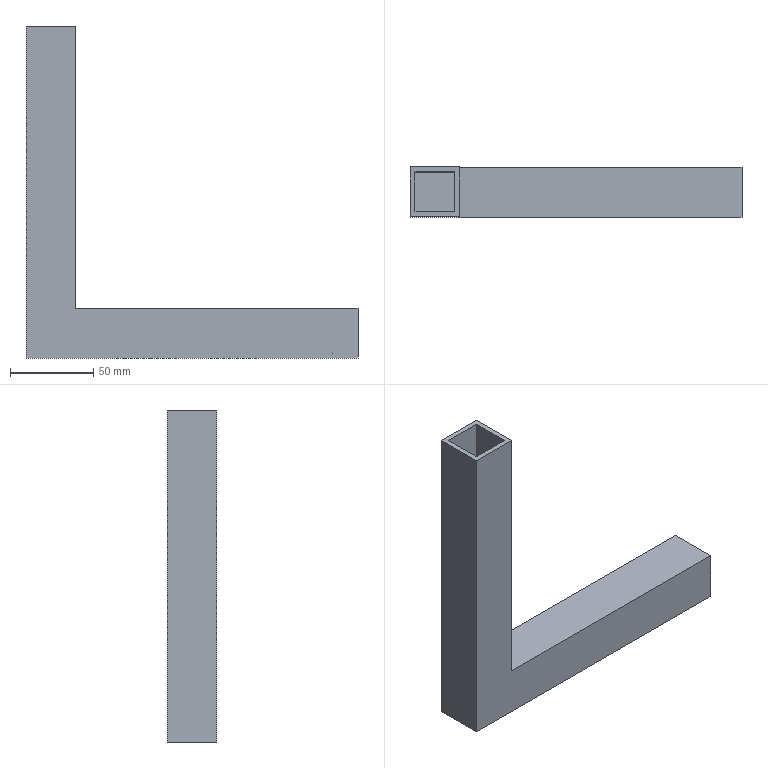Part | SolidWorks | features Extrusion 1, ICE 1, Shell 1 | 1 solid | 14 faces | box 200 x 30 x 200 mm | volume 119880 mm3 | plane 14
STEP:
#1=CARTESIAN_POINT('',(200.,0.,0.));
#2=VERTEX_POINT('',#1);
#3=CARTESIAN_POINT('',(200.,30.,0.));
#4=VERTEX_POINT('',#3);
#5=CARTESIAN_POINT('',(200.,30.,0.));
#6=DIRECTION('',(0.,1.,0.));
#7=VECTOR('',#6,1000.);
#8=LINE('',#5,#7);
#9=EDGE_CURVE('',#2,#4,#8,.T.);
#10=ORIENTED_EDGE('',*,*,#9,.F.);
#11=CARTESIAN_POINT('',(200.,0.,-30.));
#12=VERTEX_POINT('',#11);
#13=CARTESIAN_POINT('',(200.,0.,-30.));
#14=DIRECTION('',(0.,0.,1.));
#15=VECTOR('',#14,1000.);
#16=LINE('',#13,#15);
#17=EDGE_CURVE('',#12,#2,#16,.T.);
#18=ORIENTED_EDGE('',*,*,#17,.F.);
#19=CARTESIAN_POINT('',(200.,30.,-30.));
#20=VERTEX_POINT('',#19);
#21=CARTESIAN_POINT('',(200.,30.,-30.));
#22=DIRECTION('',(0.,1.,0.));
#23=VECTOR('',#22,1000.);
#24=LINE('',#21,#23);
#25=EDGE_CURVE('',#12,#20,#24,.T.);
#26=ORIENTED_EDGE('',*,*,#25,.T.);
#27=CARTESIAN_POINT('',(200.,30.,-30.));
#28=DIRECTION('',(0.,0.,1.));
#29=VECTOR('',#28,1000.);
#30=LINE('',#27,#29);
#31=EDGE_CURVE('',#20,#4,#30,.T.);
#32=ORIENTED_EDGE('',*,*,#31,.T.);
#33=EDGE_LOOP('',(#10,#18,#26,#32));
#34=FACE_OUTER_BOUND('',#33,.T.);
#35=CARTESIAN_POINT('',(200.,3.,-27.));
#36=VERTEX_POINT('',#35);
#37=CARTESIAN_POINT('',(200.,3.,-3.));
#38=VERTEX_POINT('',#37);
#39=CARTESIAN_POINT('',(200.,3.,-30.));
#40=DIRECTION('',(0.,0.,1.));
#41=VECTOR('',#40,1000.);
#42=LINE('',#39,#41);
#43=EDGE_CURVE('',#36,#38,#42,.T.);
#44=ORIENTED_EDGE('',*,*,#43,.T.);
#45=CARTESIAN_POINT('',(200.,27.,-3.));
#46=VERTEX_POINT('',#45);
#47=CARTESIAN_POINT('',(200.,30.,-3.));
#48=DIRECTION('',(0.,1.,0.));
#49=VECTOR('',#48,1000.);
#50=LINE('',#47,#49);
#51=EDGE_CURVE('',#38,#46,#50,.T.);
#52=ORIENTED_EDGE('',*,*,#51,.T.);
#53=CARTESIAN_POINT('',(200.,27.,-27.));
#54=VERTEX_POINT('',#53);
#55=CARTESIAN_POINT('',(200.,27.,-30.));
#56=DIRECTION('',(0.,0.,1.));
#57=VECTOR('',#56,1000.);
#58=LINE('',#55,#57);
#59=EDGE_CURVE('',#54,#46,#58,.T.);
#60=ORIENTED_EDGE('',*,*,#59,.F.);
#61=CARTESIAN_POINT('',(200.,30.,-27.));
#62=DIRECTION('',(0.,1.,0.));
#63=VECTOR('',#62,1000.);
#64=LINE('',#61,#63);
#65=EDGE_CURVE('',#36,#54,#64,.T.);
#66=ORIENTED_EDGE('',*,*,#65,.F.);
#67=EDGE_LOOP('',(#44,#52,#60,#66));
#68=FACE_BOUND('',#67,.T.);
#69=CARTESIAN_POINT('',(200.,30.,-30.));
#70=DIRECTION('',(1.,0.,0.));
#71=DIRECTION('',(0.,0.,-1.));
#72=AXIS2_PLACEMENT_3D('',#69,#70,#71);
#73=PLANE('',#72);
#74=ADVANCED_FACE('',(#34,#68),#73,.T.);
#75=CARTESIAN_POINT('',(0.,30.,170.));
#76=VERTEX_POINT('',#75);
#77=CARTESIAN_POINT('',(0.,0.,170.));
#78=VERTEX_POINT('',#77);
#79=CARTESIAN_POINT('',(0.,0.,170.));
#80=DIRECTION('',(0.,-1.,0.));
#81=VECTOR('',#80,1000.);
#82=LINE('',#79,#81);
#83=EDGE_CURVE('',#76,#78,#82,.T.);
#84=ORIENTED_EDGE('',*,*,#83,.T.);
#85=CARTESIAN_POINT('',(30.,0.,170.));
#86=VERTEX_POINT('',#85);
#87=CARTESIAN_POINT('',(30.,0.,170.));
#88=DIRECTION('',(1.,0.,0.));
#89=VECTOR('',#88,1000.);
#90=LINE('',#87,#89);
#91=EDGE_CURVE('',#78,#86,#90,.T.);
#92=ORIENTED_EDGE('',*,*,#91,.T.);
#93=CARTESIAN_POINT('',(30.,30.,170.));
#94=VERTEX_POINT('',#93);
#95=CARTESIAN_POINT('',(30.,30.,170.));
#96=DIRECTION('',(0.,1.,0.));
#97=VECTOR('',#96,1000.);
#98=LINE('',#95,#97);
#99=EDGE_CURVE('',#86,#94,#98,.T.);
#100=ORIENTED_EDGE('',*,*,#99,.T.);
#101=CARTESIAN_POINT('',(0.,30.,170.));
#102=DIRECTION('',(-1.,0.,0.));
#103=VECTOR('',#102,1000.);
#104=LINE('',#101,#103);
#105=EDGE_CURVE('',#94,#76,#104,.T.);
#106=ORIENTED_EDGE('',*,*,#105,.T.);
#107=EDGE_LOOP('',(#84,#92,#100,#106));
#108=FACE_OUTER_BOUND('',#107,.T.);
#109=CARTESIAN_POINT('',(3.,27.,170.));
#110=VERTEX_POINT('',#109);
#111=CARTESIAN_POINT('',(3.,3.,170.));
#112=VERTEX_POINT('',#111);
#113=CARTESIAN_POINT('',(3.,0.,170.));
#114=DIRECTION('',(0.,-1.,0.));
#115=VECTOR('',#114,1000.);
#116=LINE('',#113,#115);
#117=EDGE_CURVE('',#110,#112,#116,.T.);
#118=ORIENTED_EDGE('',*,*,#117,.F.);
#119=CARTESIAN_POINT('',(27.,27.,170.));
#120=VERTEX_POINT('',#119);
#121=CARTESIAN_POINT('',(0.,27.,170.));
#122=DIRECTION('',(-1.,0.,0.));
#123=VECTOR('',#122,1000.);
#124=LINE('',#121,#123);
#125=EDGE_CURVE('',#120,#110,#124,.T.);
#126=ORIENTED_EDGE('',*,*,#125,.F.);
#127=CARTESIAN_POINT('',(27.,3.,170.));
#128=VERTEX_POINT('',#127);
#129=CARTESIAN_POINT('',(27.,0.,170.));
#130=DIRECTION('',(0.,1.,0.));
#131=VECTOR('',#130,1000.);
#132=LINE('',#129,#131);
#133=EDGE_CURVE('',#128,#120,#132,.T.);
#134=ORIENTED_EDGE('',*,*,#133,.F.);
#135=CARTESIAN_POINT('',(200.,3.,170.));
#136=DIRECTION('',(1.,0.,0.));
#137=VECTOR('',#136,1000.);
#138=LINE('',#135,#137);
#139=EDGE_CURVE('',#112,#128,#138,.T.);
#140=ORIENTED_EDGE('',*,*,#139,.F.);
#141=EDGE_LOOP('',(#118,#126,#134,#140));
#142=FACE_BOUND('',#141,.T.);
#143=CARTESIAN_POINT('',(0.,0.,170.));
#144=DIRECTION('',(0.,0.,-1.));
#145=DIRECTION('',(-1.,0.,0.));
#146=AXIS2_PLACEMENT_3D('',#143,#144,#145);
#147=PLANE('',#146);
#148=ADVANCED_FACE('',(#108,#142),#147,.F.);
#149=CARTESIAN_POINT('',(30.,0.,0.));
#150=VERTEX_POINT('',#149);
#151=CARTESIAN_POINT('',(30.,30.,0.));
#152=VERTEX_POINT('',#151);
#153=CARTESIAN_POINT('',(30.,30.,0.));
#154=DIRECTION('',(0.,1.,0.));
#155=VECTOR('',#154,1000.);
#156=LINE('',#153,#155);
#157=EDGE_CURVE('',#150,#152,#156,.T.);
#158=ORIENTED_EDGE('',*,*,#157,.F.);
#159=CARTESIAN_POINT('',(200.,0.,0.));
#160=DIRECTION('',(1.,0.,0.));
#161=VECTOR('',#160,1000.);
#162=LINE('',#159,#161);
#163=EDGE_CURVE('',#150,#2,#162,.T.);
#164=ORIENTED_EDGE('',*,*,#163,.T.);
#165=ORIENTED_EDGE('',*,*,#9,.T.);
#166=CARTESIAN_POINT('',(0.,30.,0.));
#167=DIRECTION('',(-1.,0.,0.));
#168=VECTOR('',#167,1000.);
#169=LINE('',#166,#168);
#170=EDGE_CURVE('',#4,#152,#169,.T.);
#171=ORIENTED_EDGE('',*,*,#170,.T.);
#172=EDGE_LOOP('',(#158,#164,#165,#171));
#173=FACE_OUTER_BOUND('',#172,.T.);
#174=CARTESIAN_POINT('',(0.,0.,0.));
#175=DIRECTION('',(0.,0.,-1.));
#176=DIRECTION('',(-1.,0.,0.));
#177=AXIS2_PLACEMENT_3D('',#174,#175,#176);
#178=PLANE('',#177);
#179=ADVANCED_FACE('',(#173),#178,.F.);
#180=ORIENTED_EDGE('',*,*,#163,.F.);
#181=CARTESIAN_POINT('',(30.,0.,170.));
#182=DIRECTION('',(0.,0.,-1.));
#183=VECTOR('',#182,1000.);
#184=LINE('',#181,#183);
#185=EDGE_CURVE('',#86,#150,#184,.T.);
#186=ORIENTED_EDGE('',*,*,#185,.F.);
#187=ORIENTED_EDGE('',*,*,#91,.F.);
#188=CARTESIAN_POINT('',(0.,0.,-30.));
#189=VERTEX_POINT('',#188);
#190=CARTESIAN_POINT('',(0.,0.,-30.));
#191=DIRECTION('',(0.,0.,1.));
#192=VECTOR('',#191,1000.);
#193=LINE('',#190,#192);
#194=EDGE_CURVE('',#189,#78,#193,.T.);
#195=ORIENTED_EDGE('',*,*,#194,.F.);
#196=CARTESIAN_POINT('',(200.,0.,-30.));
#197=DIRECTION('',(1.,0.,0.));
#198=VECTOR('',#197,1000.);
#199=LINE('',#196,#198);
#200=EDGE_CURVE('',#189,#12,#199,.T.);
#201=ORIENTED_EDGE('',*,*,#200,.T.);
#202=ORIENTED_EDGE('',*,*,#17,.T.);
#203=EDGE_LOOP('',(#180,#186,#187,#195,#201,#202));
#204=FACE_OUTER_BOUND('',#203,.T.);
#205=CARTESIAN_POINT('',(200.,0.,-30.));
#206=DIRECTION('',(0.,-1.,0.));
#207=DIRECTION('',(0.,0.,-1.));
#208=AXIS2_PLACEMENT_3D('',#205,#206,#207);
#209=PLANE('',#208);
#210=ADVANCED_FACE('',(#204),#209,.T.);
#211=ORIENTED_EDGE('',*,*,#194,.T.);
#212=ORIENTED_EDGE('',*,*,#83,.F.);
#213=CARTESIAN_POINT('',(0.,30.,-30.));
#214=VERTEX_POINT('',#213);
#215=CARTESIAN_POINT('',(0.,30.,-30.));
#216=DIRECTION('',(0.,0.,1.));
#217=VECTOR('',#216,1000.);
#218=LINE('',#215,#217);
#219=EDGE_CURVE('',#214,#76,#218,.T.);
#220=ORIENTED_EDGE('',*,*,#219,.F.);
#221=CARTESIAN_POINT('',(0.,0.,-30.));
#222=DIRECTION('',(0.,-1.,0.));
#223=VECTOR('',#222,1000.);
#224=LINE('',#221,#223);
#225=EDGE_CURVE('',#214,#189,#224,.T.);
#226=ORIENTED_EDGE('',*,*,#225,.T.);
#227=EDGE_LOOP('',(#211,#212,#220,#226));
#228=FACE_OUTER_BOUND('',#227,.T.);
#229=CARTESIAN_POINT('',(0.,0.,-30.));
#230=DIRECTION('',(-1.,0.,0.));
#231=DIRECTION('',(0.,0.,1.));
#232=AXIS2_PLACEMENT_3D('',#229,#230,#231);
#233=PLANE('',#232);
#234=ADVANCED_FACE('',(#228),#233,.T.);
#235=ORIENTED_EDGE('',*,*,#170,.F.);
#236=ORIENTED_EDGE('',*,*,#31,.F.);
#237=CARTESIAN_POINT('',(0.,30.,-30.));
#238=DIRECTION('',(-1.,0.,0.));
#239=VECTOR('',#238,1000.);
#240=LINE('',#237,#239);
#241=EDGE_CURVE('',#20,#214,#240,.T.);
#242=ORIENTED_EDGE('',*,*,#241,.T.);
#243=ORIENTED_EDGE('',*,*,#219,.T.);
#244=ORIENTED_EDGE('',*,*,#105,.F.);
#245=CARTESIAN_POINT('',(30.,30.,170.));
#246=DIRECTION('',(0.,0.,-1.));
#247=VECTOR('',#246,1000.);
#248=LINE('',#245,#247);
#249=EDGE_CURVE('',#94,#152,#248,.T.);
#250=ORIENTED_EDGE('',*,*,#249,.T.);
#251=EDGE_LOOP('',(#235,#236,#242,#243,#244,#250));
#252=FACE_OUTER_BOUND('',#251,.T.);
#253=CARTESIAN_POINT('',(0.,30.,-30.));
#254=DIRECTION('',(0.,1.,0.));
#255=DIRECTION('',(0.,0.,1.));
#256=AXIS2_PLACEMENT_3D('',#253,#254,#255);
#257=PLANE('',#256);
#258=ADVANCED_FACE('',(#252),#257,.T.);
#259=ORIENTED_EDGE('',*,*,#200,.F.);
#260=ORIENTED_EDGE('',*,*,#225,.F.);
#261=ORIENTED_EDGE('',*,*,#241,.F.);
#262=ORIENTED_EDGE('',*,*,#25,.F.);
#263=EDGE_LOOP('',(#259,#260,#261,#262));
#264=FACE_OUTER_BOUND('',#263,.T.);
#265=CARTESIAN_POINT('',(0.,0.,-30.));
#266=DIRECTION('',(0.,0.,-1.));
#267=DIRECTION('',(-1.,0.,0.));
#268=AXIS2_PLACEMENT_3D('',#265,#266,#267);
#269=PLANE('',#268);
#270=ADVANCED_FACE('',(#264),#269,.T.);
#271=ORIENTED_EDGE('',*,*,#157,.T.);
#272=ORIENTED_EDGE('',*,*,#249,.F.);
#273=ORIENTED_EDGE('',*,*,#99,.F.);
#274=ORIENTED_EDGE('',*,*,#185,.T.);
#275=EDGE_LOOP('',(#271,#272,#273,#274));
#276=FACE_OUTER_BOUND('',#275,.T.);
#277=CARTESIAN_POINT('',(30.,30.,170.));
#278=DIRECTION('',(-1.,0.,0.));
#279=DIRECTION('',(0.,0.,1.));
#280=AXIS2_PLACEMENT_3D('',#277,#278,#279);
#281=PLANE('',#280);
#282=ADVANCED_FACE('',(#276),#281,.F.);
#283=CARTESIAN_POINT('',(27.,3.,-3.));
#284=VERTEX_POINT('',#283);
#285=CARTESIAN_POINT('',(27.,27.,-3.));
#286=VERTEX_POINT('',#285);
#287=CARTESIAN_POINT('',(27.,0.,-3.));
#288=DIRECTION('',(0.,1.,0.));
#289=VECTOR('',#288,1000.);
#290=LINE('',#287,#289);
#291=EDGE_CURVE('',#284,#286,#290,.T.);
#292=ORIENTED_EDGE('',*,*,#291,.T.);
#293=CARTESIAN_POINT('',(0.,27.,-3.));
#294=DIRECTION('',(-1.,0.,0.));
#295=VECTOR('',#294,1000.);
#296=LINE('',#293,#295);
#297=EDGE_CURVE('',#46,#286,#296,.T.);
#298=ORIENTED_EDGE('',*,*,#297,.F.);
#299=ORIENTED_EDGE('',*,*,#51,.F.);
#300=CARTESIAN_POINT('',(200.,3.,-3.));
#301=DIRECTION('',(1.,0.,0.));
#302=VECTOR('',#301,1000.);
#303=LINE('',#300,#302);
#304=EDGE_CURVE('',#284,#38,#303,.T.);
#305=ORIENTED_EDGE('',*,*,#304,.F.);
#306=EDGE_LOOP('',(#292,#298,#299,#305));
#307=FACE_OUTER_BOUND('',#306,.T.);
#308=CARTESIAN_POINT('',(0.,0.,-3.));
#309=DIRECTION('',(0.,0.,-1.));
#310=DIRECTION('',(-1.,0.,0.));
#311=AXIS2_PLACEMENT_3D('',#308,#309,#310);
#312=PLANE('',#311);
#313=ADVANCED_FACE('',(#307),#312,.T.);
#314=ORIENTED_EDGE('',*,*,#304,.T.);
#315=ORIENTED_EDGE('',*,*,#43,.F.);
#316=CARTESIAN_POINT('',(3.,3.,-27.));
#317=VERTEX_POINT('',#316);
#318=CARTESIAN_POINT('',(200.,3.,-27.));
#319=DIRECTION('',(1.,0.,0.));
#320=VECTOR('',#319,1000.);
#321=LINE('',#318,#320);
#322=EDGE_CURVE('',#317,#36,#321,.T.);
#323=ORIENTED_EDGE('',*,*,#322,.F.);
#324=CARTESIAN_POINT('',(3.,3.,-30.));
#325=DIRECTION('',(0.,0.,1.));
#326=VECTOR('',#325,1000.);
#327=LINE('',#324,#326);
#328=EDGE_CURVE('',#317,#112,#327,.T.);
#329=ORIENTED_EDGE('',*,*,#328,.T.);
#330=ORIENTED_EDGE('',*,*,#139,.T.);
#331=CARTESIAN_POINT('',(27.,3.,-30.));
#332=DIRECTION('',(0.,0.,-1.));
#333=VECTOR('',#332,1000.);
#334=LINE('',#331,#333);
#335=EDGE_CURVE('',#128,#284,#334,.T.);
#336=ORIENTED_EDGE('',*,*,#335,.T.);
#337=EDGE_LOOP('',(#314,#315,#323,#329,#330,#336));
#338=FACE_OUTER_BOUND('',#337,.T.);
#339=CARTESIAN_POINT('',(200.,3.,-30.));
#340=DIRECTION('',(0.,-1.,0.));
#341=DIRECTION('',(0.,0.,-1.));
#342=AXIS2_PLACEMENT_3D('',#339,#340,#341);
#343=PLANE('',#342);
#344=ADVANCED_FACE('',(#338),#343,.F.);
#345=ORIENTED_EDGE('',*,*,#328,.F.);
#346=CARTESIAN_POINT('',(3.,27.,-27.));
#347=VERTEX_POINT('',#346);
#348=CARTESIAN_POINT('',(3.,0.,-27.));
#349=DIRECTION('',(0.,-1.,0.));
#350=VECTOR('',#349,1000.);
#351=LINE('',#348,#350);
#352=EDGE_CURVE('',#347,#317,#351,.T.);
#353=ORIENTED_EDGE('',*,*,#352,.F.);
#354=CARTESIAN_POINT('',(3.,27.,-30.));
#355=DIRECTION('',(0.,0.,1.));
#356=VECTOR('',#355,1000.);
#357=LINE('',#354,#356);
#358=EDGE_CURVE('',#347,#110,#357,.T.);
#359=ORIENTED_EDGE('',*,*,#358,.T.);
#360=ORIENTED_EDGE('',*,*,#117,.T.);
#361=EDGE_LOOP('',(#345,#353,#359,#360));
#362=FACE_OUTER_BOUND('',#361,.T.);
#363=CARTESIAN_POINT('',(3.,0.,-30.));
#364=DIRECTION('',(-1.,0.,0.));
#365=DIRECTION('',(0.,0.,1.));
#366=AXIS2_PLACEMENT_3D('',#363,#364,#365);
#367=PLANE('',#366);
#368=ADVANCED_FACE('',(#362),#367,.F.);
#369=ORIENTED_EDGE('',*,*,#297,.T.);
#370=CARTESIAN_POINT('',(27.,27.,170.));
#371=DIRECTION('',(0.,0.,-1.));
#372=VECTOR('',#371,1000.);
#373=LINE('',#370,#372);
#374=EDGE_CURVE('',#120,#286,#373,.T.);
#375=ORIENTED_EDGE('',*,*,#374,.F.);
#376=ORIENTED_EDGE('',*,*,#125,.T.);
#377=ORIENTED_EDGE('',*,*,#358,.F.);
#378=CARTESIAN_POINT('',(0.,27.,-27.));
#379=DIRECTION('',(-1.,0.,0.));
#380=VECTOR('',#379,1000.);
#381=LINE('',#378,#380);
#382=EDGE_CURVE('',#54,#347,#381,.T.);
#383=ORIENTED_EDGE('',*,*,#382,.F.);
#384=ORIENTED_EDGE('',*,*,#59,.T.);
#385=EDGE_LOOP('',(#369,#375,#376,#377,#383,#384));
#386=FACE_OUTER_BOUND('',#385,.T.);
#387=CARTESIAN_POINT('',(0.,27.,-30.));
#388=DIRECTION('',(0.,1.,0.));
#389=DIRECTION('',(0.,0.,1.));
#390=AXIS2_PLACEMENT_3D('',#387,#388,#389);
#391=PLANE('',#390);
#392=ADVANCED_FACE('',(#386),#391,.F.);
#393=ORIENTED_EDGE('',*,*,#322,.T.);
#394=ORIENTED_EDGE('',*,*,#65,.T.);
#395=ORIENTED_EDGE('',*,*,#382,.T.);
#396=ORIENTED_EDGE('',*,*,#352,.T.);
#397=EDGE_LOOP('',(#393,#394,#395,#396));
#398=FACE_OUTER_BOUND('',#397,.T.);
#399=CARTESIAN_POINT('',(0.,0.,-27.));
#400=DIRECTION('',(0.,0.,-1.));
#401=DIRECTION('',(-1.,0.,0.));
#402=AXIS2_PLACEMENT_3D('',#399,#400,#401);
#403=PLANE('',#402);
#404=ADVANCED_FACE('',(#398),#403,.F.);
#405=ORIENTED_EDGE('',*,*,#291,.F.);
#406=ORIENTED_EDGE('',*,*,#335,.F.);
#407=ORIENTED_EDGE('',*,*,#133,.T.);
#408=ORIENTED_EDGE('',*,*,#374,.T.);
#409=EDGE_LOOP('',(#405,#406,#407,#408));
#410=FACE_OUTER_BOUND('',#409,.T.);
#411=CARTESIAN_POINT('',(27.,30.,170.));
#412=DIRECTION('',(-1.,0.,0.));
#413=DIRECTION('',(0.,0.,1.));
#414=AXIS2_PLACEMENT_3D('',#411,#412,#413);
#415=PLANE('',#414);
#416=ADVANCED_FACE('',(#410),#415,.T.);
#417=CLOSED_SHELL('',(#74,#148,#179,#210,#234,#258,#270,#282,#313,#344,#368,#392,#404,#416));
#418=MANIFOLD_SOLID_BREP('',#417);
#419=CARTESIAN_POINT('',(0.,0.,0.));
#420=DIRECTION('',(0.,0.,1.));
#421=DIRECTION('',(1.,0.,0.));
#422=AXIS2_PLACEMENT_3D('',#419,#420,#421);
#423=(LENGTH_UNIT()NAMED_UNIT(*)SI_UNIT(.MILLI.,.METRE.));
#424=UNCERTAINTY_MEASURE_WITH_UNIT(LENGTH_MEASURE(0.00001),#423,'','');
#425=(NAMED_UNIT(*)PLANE_ANGLE_UNIT()SI_UNIT($,.RADIAN.));
#426=(NAMED_UNIT(*)SI_UNIT($,.STERADIAN.)SOLID_ANGLE_UNIT());
#427=(GEOMETRIC_REPRESENTATION_CONTEXT(3)GLOBAL_UNCERTAINTY_ASSIGNED_CONTEXT((#424))GLOBAL_UNIT_ASSIGNED_CONTEXT((#423,#425,#426))REPRESENTATION_CONTEXT('',''));
#428=ADVANCED_BREP_SHAPE_REPRESENTATION('',(#418,#422),#427);